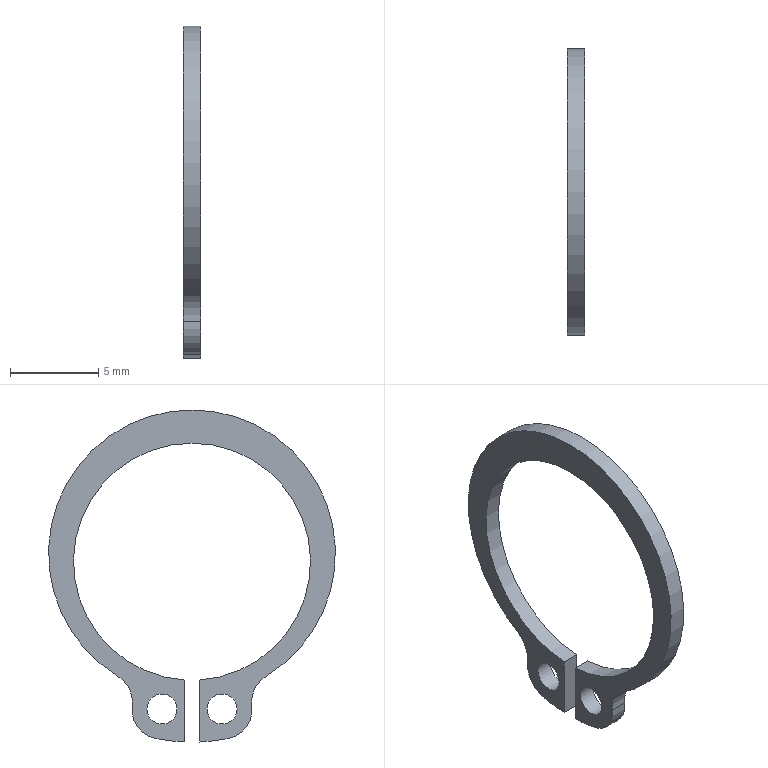Part | NX | features DATUM_CSYS 2, EXTRUDE 1, SKETCH 1 | 1 solid | 14 faces | box 1 x 16.22 x 18.771 mm | volume 75.444 mm3 | cylinder 10 | plane 4 | commonest cylinder face diameters 3.4 x4 1.7 x2 20.4 x2 13.4 x1 16.22 x1
STEP:
#1=CARTESIAN_POINT('',(0.,-4.196,-6.94));
#2=VERTEX_POINT('',#1);
#3=CARTESIAN_POINT('',(0.,-3.388,-8.596));
#4=VERTEX_POINT('',#3);
#5=CARTESIAN_POINT('',(0.,-5.076,-8.395));
#6=DIRECTION('',(-1.,0.,0.));
#7=DIRECTION('',(0.,1.,0.));
#8=AXIS2_PLACEMENT_3D('',#5,#6,#7);
#9=CIRCLE('',#8,1.7);
#10=EDGE_CURVE('',#2,#4,#9,.T.);
#11=ORIENTED_EDGE('',*,*,#10,.T.);
#12=CARTESIAN_POINT('',(1.,-3.388,-8.596));
#13=VERTEX_POINT('',#12);
#14=CARTESIAN_POINT('',(1.,-3.388,-8.596));
#15=DIRECTION('',(-1.,0.,0.));
#16=VECTOR('',#15,1000.);
#17=LINE('',#14,#16);
#18=EDGE_CURVE('',#13,#4,#17,.T.);
#19=ORIENTED_EDGE('',*,*,#18,.F.);
#20=CARTESIAN_POINT('',(1.,-4.196,-6.94));
#21=VERTEX_POINT('',#20);
#22=CARTESIAN_POINT('',(1.,-5.076,-8.395));
#23=DIRECTION('',(-1.,0.,0.));
#24=DIRECTION('',(0.,1.,0.));
#25=AXIS2_PLACEMENT_3D('',#22,#23,#24);
#26=CIRCLE('',#25,1.7);
#27=EDGE_CURVE('',#21,#13,#26,.T.);
#28=ORIENTED_EDGE('',*,*,#27,.F.);
#29=CARTESIAN_POINT('',(1.,-4.196,-6.94));
#30=DIRECTION('',(-1.,0.,0.));
#31=VECTOR('',#30,1000.);
#32=LINE('',#29,#31);
#33=EDGE_CURVE('',#21,#2,#32,.T.);
#34=ORIENTED_EDGE('',*,*,#33,.T.);
#35=EDGE_LOOP('',(#11,#19,#28,#34));
#36=FACE_BOUND('',#35,.T.);
#37=CARTESIAN_POINT('',(1.,-5.076,-8.395));
#38=DIRECTION('',(-1.,0.,0.));
#39=DIRECTION('',(0.,0.,1.));
#40=AXIS2_PLACEMENT_3D('',#37,#38,#39);
#41=CYLINDRICAL_SURFACE('',#40,1.7);
#42=ADVANCED_FACE('',(#36),#41,.F.);
#43=CARTESIAN_POINT('',(0.,-2.04,-10.464));
#44=VERTEX_POINT('',#43);
#45=CARTESIAN_POINT('',(0.,-1.7,-8.798));
#46=DIRECTION('',(1.,0.,0.));
#47=DIRECTION('',(0.,1.,0.));
#48=AXIS2_PLACEMENT_3D('',#45,#46,#47);
#49=CIRCLE('',#48,1.7);
#50=EDGE_CURVE('',#4,#44,#49,.T.);
#51=ORIENTED_EDGE('',*,*,#50,.T.);
#52=CARTESIAN_POINT('',(1.,-2.04,-10.464));
#53=VERTEX_POINT('',#52);
#54=CARTESIAN_POINT('',(1.,-2.04,-10.464));
#55=DIRECTION('',(-1.,0.,0.));
#56=VECTOR('',#55,1000.);
#57=LINE('',#54,#56);
#58=EDGE_CURVE('',#53,#44,#57,.T.);
#59=ORIENTED_EDGE('',*,*,#58,.F.);
#60=CARTESIAN_POINT('',(1.,-1.7,-8.798));
#61=DIRECTION('',(1.,0.,0.));
#62=DIRECTION('',(0.,1.,0.));
#63=AXIS2_PLACEMENT_3D('',#60,#61,#62);
#64=CIRCLE('',#63,1.7);
#65=EDGE_CURVE('',#13,#53,#64,.T.);
#66=ORIENTED_EDGE('',*,*,#65,.F.);
#67=ORIENTED_EDGE('',*,*,#18,.T.);
#68=EDGE_LOOP('',(#51,#59,#66,#67));
#69=FACE_BOUND('',#68,.T.);
#70=CARTESIAN_POINT('',(1.,-1.7,-8.798));
#71=DIRECTION('',(-1.,0.,0.));
#72=DIRECTION('',(0.,0.,1.));
#73=AXIS2_PLACEMENT_3D('',#70,#71,#72);
#74=CYLINDRICAL_SURFACE('',#73,1.7);
#75=ADVANCED_FACE('',(#69),#74,.T.);
#76=CARTESIAN_POINT('',(0.,-0.425,-10.661));
#77=VERTEX_POINT('',#76);
#78=CARTESIAN_POINT('',(0.,0.,-0.47));
#79=DIRECTION('',(1.,0.,0.));
#80=DIRECTION('',(0.,1.,0.));
#81=AXIS2_PLACEMENT_3D('',#78,#79,#80);
#82=CIRCLE('',#81,10.2);
#83=EDGE_CURVE('',#44,#77,#82,.T.);
#84=ORIENTED_EDGE('',*,*,#83,.T.);
#85=CARTESIAN_POINT('',(1.,-0.425,-10.661));
#86=VERTEX_POINT('',#85);
#87=CARTESIAN_POINT('',(1.,-0.425,-10.661));
#88=DIRECTION('',(-1.,0.,0.));
#89=VECTOR('',#88,1000.);
#90=LINE('',#87,#89);
#91=EDGE_CURVE('',#86,#77,#90,.T.);
#92=ORIENTED_EDGE('',*,*,#91,.F.);
#93=CARTESIAN_POINT('',(1.,0.,-0.47));
#94=DIRECTION('',(1.,0.,0.));
#95=DIRECTION('',(0.,1.,0.));
#96=AXIS2_PLACEMENT_3D('',#93,#94,#95);
#97=CIRCLE('',#96,10.2);
#98=EDGE_CURVE('',#53,#86,#97,.T.);
#99=ORIENTED_EDGE('',*,*,#98,.F.);
#100=ORIENTED_EDGE('',*,*,#58,.T.);
#101=EDGE_LOOP('',(#84,#92,#99,#100));
#102=FACE_BOUND('',#101,.T.);
#103=CARTESIAN_POINT('',(1.,0.,-0.47));
#104=DIRECTION('',(-1.,0.,0.));
#105=DIRECTION('',(0.,0.,1.));
#106=AXIS2_PLACEMENT_3D('',#103,#104,#105);
#107=CYLINDRICAL_SURFACE('',#106,10.2);
#108=ADVANCED_FACE('',(#102),#107,.T.);
#109=CARTESIAN_POINT('',(0.,-0.425,-7.157));
#110=VERTEX_POINT('',#109);
#111=CARTESIAN_POINT('',(0.,-0.425,-10.661));
#112=DIRECTION('',(0.,0.,1.));
#113=VECTOR('',#112,1000.);
#114=LINE('',#111,#113);
#115=EDGE_CURVE('',#77,#110,#114,.T.);
#116=ORIENTED_EDGE('',*,*,#115,.T.);
#117=CARTESIAN_POINT('',(1.,-0.425,-7.157));
#118=VERTEX_POINT('',#117);
#119=CARTESIAN_POINT('',(1.,-0.425,-7.157));
#120=DIRECTION('',(-1.,0.,0.));
#121=VECTOR('',#120,1000.);
#122=LINE('',#119,#121);
#123=EDGE_CURVE('',#118,#110,#122,.T.);
#124=ORIENTED_EDGE('',*,*,#123,.F.);
#125=CARTESIAN_POINT('',(1.,-0.425,-10.661));
#126=DIRECTION('',(0.,0.,1.));
#127=VECTOR('',#126,1000.);
#128=LINE('',#125,#127);
#129=EDGE_CURVE('',#86,#118,#128,.T.);
#130=ORIENTED_EDGE('',*,*,#129,.F.);
#131=ORIENTED_EDGE('',*,*,#91,.T.);
#132=EDGE_LOOP('',(#116,#124,#130,#131));
#133=FACE_BOUND('',#132,.T.);
#134=CARTESIAN_POINT('',(1.,-0.425,-10.661));
#135=DIRECTION('',(0.,-1.,0.));
#136=DIRECTION('',(0.,0.,-1.));
#137=AXIS2_PLACEMENT_3D('',#134,#135,#136);
#138=PLANE('',#137);
#139=ADVANCED_FACE('',(#133),#138,.F.);
#140=CARTESIAN_POINT('',(0.,0.425,-7.157));
#141=VERTEX_POINT('',#140);
#142=CARTESIAN_POINT('',(0.,0.,-0.47));
#143=DIRECTION('',(-1.,0.,0.));
#144=DIRECTION('',(0.,1.,0.));
#145=AXIS2_PLACEMENT_3D('',#142,#143,#144);
#146=CIRCLE('',#145,6.7);
#147=EDGE_CURVE('',#110,#141,#146,.T.);
#148=ORIENTED_EDGE('',*,*,#147,.T.);
#149=CARTESIAN_POINT('',(1.,0.425,-7.157));
#150=VERTEX_POINT('',#149);
#151=CARTESIAN_POINT('',(1.,0.425,-7.157));
#152=DIRECTION('',(-1.,0.,0.));
#153=VECTOR('',#152,1000.);
#154=LINE('',#151,#153);
#155=EDGE_CURVE('',#150,#141,#154,.T.);
#156=ORIENTED_EDGE('',*,*,#155,.F.);
#157=CARTESIAN_POINT('',(1.,0.,-0.47));
#158=DIRECTION('',(-1.,0.,0.));
#159=DIRECTION('',(0.,1.,0.));
#160=AXIS2_PLACEMENT_3D('',#157,#158,#159);
#161=CIRCLE('',#160,6.7);
#162=EDGE_CURVE('',#118,#150,#161,.T.);
#163=ORIENTED_EDGE('',*,*,#162,.F.);
#164=ORIENTED_EDGE('',*,*,#123,.T.);
#165=EDGE_LOOP('',(#148,#156,#163,#164));
#166=FACE_BOUND('',#165,.T.);
#167=CARTESIAN_POINT('',(1.,0.,-0.47));
#168=DIRECTION('',(-1.,0.,0.));
#169=DIRECTION('',(0.,0.,1.));
#170=AXIS2_PLACEMENT_3D('',#167,#168,#169);
#171=CYLINDRICAL_SURFACE('',#170,6.7);
#172=ADVANCED_FACE('',(#166),#171,.F.);
#173=CARTESIAN_POINT('',(0.,0.425,-10.661));
#174=VERTEX_POINT('',#173);
#175=CARTESIAN_POINT('',(0.,0.425,-7.157));
#176=DIRECTION('',(0.,0.,-1.));
#177=VECTOR('',#176,1000.);
#178=LINE('',#175,#177);
#179=EDGE_CURVE('',#141,#174,#178,.T.);
#180=ORIENTED_EDGE('',*,*,#179,.T.);
#181=CARTESIAN_POINT('',(1.,0.425,-10.661));
#182=VERTEX_POINT('',#181);
#183=CARTESIAN_POINT('',(1.,0.425,-10.661));
#184=DIRECTION('',(-1.,0.,0.));
#185=VECTOR('',#184,1000.);
#186=LINE('',#183,#185);
#187=EDGE_CURVE('',#182,#174,#186,.T.);
#188=ORIENTED_EDGE('',*,*,#187,.F.);
#189=CARTESIAN_POINT('',(1.,0.425,-7.157));
#190=DIRECTION('',(0.,0.,-1.));
#191=VECTOR('',#190,1000.);
#192=LINE('',#189,#191);
#193=EDGE_CURVE('',#150,#182,#192,.T.);
#194=ORIENTED_EDGE('',*,*,#193,.F.);
#195=ORIENTED_EDGE('',*,*,#155,.T.);
#196=EDGE_LOOP('',(#180,#188,#194,#195));
#197=FACE_BOUND('',#196,.T.);
#198=CARTESIAN_POINT('',(1.,0.425,-7.157));
#199=DIRECTION('',(0.,1.,0.));
#200=DIRECTION('',(0.,0.,1.));
#201=AXIS2_PLACEMENT_3D('',#198,#199,#200);
#202=PLANE('',#201);
#203=ADVANCED_FACE('',(#197),#202,.F.);
#204=CARTESIAN_POINT('',(0.,2.04,-10.464));
#205=VERTEX_POINT('',#204);
#206=CARTESIAN_POINT('',(0.,0.,-0.47));
#207=DIRECTION('',(1.,0.,0.));
#208=DIRECTION('',(0.,1.,0.));
#209=AXIS2_PLACEMENT_3D('',#206,#207,#208);
#210=CIRCLE('',#209,10.2);
#211=EDGE_CURVE('',#174,#205,#210,.T.);
#212=ORIENTED_EDGE('',*,*,#211,.T.);
#213=CARTESIAN_POINT('',(1.,2.04,-10.464));
#214=VERTEX_POINT('',#213);
#215=CARTESIAN_POINT('',(1.,2.04,-10.464));
#216=DIRECTION('',(-1.,0.,0.));
#217=VECTOR('',#216,1000.);
#218=LINE('',#215,#217);
#219=EDGE_CURVE('',#214,#205,#218,.T.);
#220=ORIENTED_EDGE('',*,*,#219,.F.);
#221=CARTESIAN_POINT('',(1.,0.,-0.47));
#222=DIRECTION('',(1.,0.,0.));
#223=DIRECTION('',(0.,1.,0.));
#224=AXIS2_PLACEMENT_3D('',#221,#222,#223);
#225=CIRCLE('',#224,10.2);
#226=EDGE_CURVE('',#182,#214,#225,.T.);
#227=ORIENTED_EDGE('',*,*,#226,.F.);
#228=ORIENTED_EDGE('',*,*,#187,.T.);
#229=EDGE_LOOP('',(#212,#220,#227,#228));
#230=FACE_BOUND('',#229,.T.);
#231=CARTESIAN_POINT('',(1.,0.,-0.47));
#232=DIRECTION('',(-1.,0.,0.));
#233=DIRECTION('',(0.,0.,1.));
#234=AXIS2_PLACEMENT_3D('',#231,#232,#233);
#235=CYLINDRICAL_SURFACE('',#234,10.2);
#236=ADVANCED_FACE('',(#230),#235,.T.);
#237=CARTESIAN_POINT('',(0.,3.388,-8.596));
#238=VERTEX_POINT('',#237);
#239=CARTESIAN_POINT('',(0.,1.7,-8.798));
#240=DIRECTION('',(1.,0.,0.));
#241=DIRECTION('',(0.,-1.,0.));
#242=AXIS2_PLACEMENT_3D('',#239,#240,#241);
#243=CIRCLE('',#242,1.7);
#244=EDGE_CURVE('',#205,#238,#243,.T.);
#245=ORIENTED_EDGE('',*,*,#244,.T.);
#246=CARTESIAN_POINT('',(1.,3.388,-8.596));
#247=VERTEX_POINT('',#246);
#248=CARTESIAN_POINT('',(1.,3.388,-8.596));
#249=DIRECTION('',(-1.,0.,0.));
#250=VECTOR('',#249,1000.);
#251=LINE('',#248,#250);
#252=EDGE_CURVE('',#247,#238,#251,.T.);
#253=ORIENTED_EDGE('',*,*,#252,.F.);
#254=CARTESIAN_POINT('',(1.,1.7,-8.798));
#255=DIRECTION('',(1.,0.,0.));
#256=DIRECTION('',(0.,-1.,0.));
#257=AXIS2_PLACEMENT_3D('',#254,#255,#256);
#258=CIRCLE('',#257,1.7);
#259=EDGE_CURVE('',#214,#247,#258,.T.);
#260=ORIENTED_EDGE('',*,*,#259,.F.);
#261=ORIENTED_EDGE('',*,*,#219,.T.);
#262=EDGE_LOOP('',(#245,#253,#260,#261));
#263=FACE_BOUND('',#262,.T.);
#264=CARTESIAN_POINT('',(1.,1.7,-8.798));
#265=DIRECTION('',(-1.,0.,0.));
#266=DIRECTION('',(0.,0.,1.));
#267=AXIS2_PLACEMENT_3D('',#264,#265,#266);
#268=CYLINDRICAL_SURFACE('',#267,1.7);
#269=ADVANCED_FACE('',(#263),#268,.T.);
#270=CARTESIAN_POINT('',(0.,4.196,-6.94));
#271=VERTEX_POINT('',#270);
#272=CARTESIAN_POINT('',(0.,5.076,-8.395));
#273=DIRECTION('',(-1.,0.,0.));
#274=DIRECTION('',(0.,-1.,0.));
#275=AXIS2_PLACEMENT_3D('',#272,#273,#274);
#276=CIRCLE('',#275,1.7);
#277=EDGE_CURVE('',#238,#271,#276,.T.);
#278=ORIENTED_EDGE('',*,*,#277,.T.);
#279=CARTESIAN_POINT('',(1.,4.196,-6.94));
#280=VERTEX_POINT('',#279);
#281=CARTESIAN_POINT('',(1.,4.196,-6.94));
#282=DIRECTION('',(-1.,0.,0.));
#283=VECTOR('',#282,1000.);
#284=LINE('',#281,#283);
#285=EDGE_CURVE('',#280,#271,#284,.T.);
#286=ORIENTED_EDGE('',*,*,#285,.F.);
#287=CARTESIAN_POINT('',(1.,5.076,-8.395));
#288=DIRECTION('',(-1.,0.,0.));
#289=DIRECTION('',(0.,-1.,0.));
#290=AXIS2_PLACEMENT_3D('',#287,#288,#289);
#291=CIRCLE('',#290,1.7);
#292=EDGE_CURVE('',#247,#280,#291,.T.);
#293=ORIENTED_EDGE('',*,*,#292,.F.);
#294=ORIENTED_EDGE('',*,*,#252,.T.);
#295=EDGE_LOOP('',(#278,#286,#293,#294));
#296=FACE_BOUND('',#295,.T.);
#297=CARTESIAN_POINT('',(1.,5.076,-8.395));
#298=DIRECTION('',(-1.,0.,0.));
#299=DIRECTION('',(0.,0.,1.));
#300=AXIS2_PLACEMENT_3D('',#297,#298,#299);
#301=CYLINDRICAL_SURFACE('',#300,1.7);
#302=ADVANCED_FACE('',(#296),#301,.F.);
#303=CARTESIAN_POINT('',(1.,-0.85,-8.798));
#304=VERTEX_POINT('',#303);
#305=CARTESIAN_POINT('',(1.,-1.7,-8.798));
#306=DIRECTION('',(1.,0.,0.));
#307=DIRECTION('',(0.,1.,0.));
#308=AXIS2_PLACEMENT_3D('',#305,#306,#307);
#309=CIRCLE('',#308,0.85);
#310=EDGE_CURVE('',#304,#304,#309,.T.);
#311=ORIENTED_EDGE('',*,*,#310,.T.);
#312=EDGE_LOOP('',(#311));
#313=FACE_BOUND('',#312,.T.);
#314=CARTESIAN_POINT('',(0.,-0.85,-8.798));
#315=VERTEX_POINT('',#314);
#316=CARTESIAN_POINT('',(0.,-1.7,-8.798));
#317=DIRECTION('',(1.,0.,0.));
#318=DIRECTION('',(0.,1.,0.));
#319=AXIS2_PLACEMENT_3D('',#316,#317,#318);
#320=CIRCLE('',#319,0.85);
#321=EDGE_CURVE('',#315,#315,#320,.T.);
#322=ORIENTED_EDGE('',*,*,#321,.F.);
#323=EDGE_LOOP('',(#322));
#324=FACE_BOUND('',#323,.T.);
#325=CARTESIAN_POINT('',(1.,-1.7,-8.798));
#326=DIRECTION('',(-1.,0.,0.));
#327=DIRECTION('',(0.,0.,1.));
#328=AXIS2_PLACEMENT_3D('',#325,#326,#327);
#329=CYLINDRICAL_SURFACE('',#328,0.85);
#330=ADVANCED_FACE('',(#313,#324),#329,.F.);
#331=CARTESIAN_POINT('',(0.,0.,0.));
#332=DIRECTION('',(1.,0.,0.));
#333=DIRECTION('',(0.,1.,0.));
#334=AXIS2_PLACEMENT_3D('',#331,#332,#333);
#335=CIRCLE('',#334,8.11);
#336=EDGE_CURVE('',#271,#2,#335,.T.);
#337=ORIENTED_EDGE('',*,*,#336,.T.);
#338=ORIENTED_EDGE('',*,*,#33,.F.);
#339=CARTESIAN_POINT('',(1.,0.,0.));
#340=DIRECTION('',(1.,0.,0.));
#341=DIRECTION('',(0.,1.,0.));
#342=AXIS2_PLACEMENT_3D('',#339,#340,#341);
#343=CIRCLE('',#342,8.11);
#344=EDGE_CURVE('',#280,#21,#343,.T.);
#345=ORIENTED_EDGE('',*,*,#344,.F.);
#346=ORIENTED_EDGE('',*,*,#285,.T.);
#347=EDGE_LOOP('',(#337,#338,#345,#346));
#348=FACE_BOUND('',#347,.T.);
#349=CARTESIAN_POINT('',(1.,0.,0.));
#350=DIRECTION('',(-1.,0.,0.));
#351=DIRECTION('',(0.,0.,1.));
#352=AXIS2_PLACEMENT_3D('',#349,#350,#351);
#353=CYLINDRICAL_SURFACE('',#352,8.11);
#354=ADVANCED_FACE('',(#348),#353,.T.);
#355=CARTESIAN_POINT('',(1.,2.55,-8.798));
#356=VERTEX_POINT('',#355);
#357=CARTESIAN_POINT('',(1.,1.7,-8.798));
#358=DIRECTION('',(1.,0.,0.));
#359=DIRECTION('',(0.,1.,0.));
#360=AXIS2_PLACEMENT_3D('',#357,#358,#359);
#361=CIRCLE('',#360,0.85);
#362=EDGE_CURVE('',#356,#356,#361,.T.);
#363=ORIENTED_EDGE('',*,*,#362,.T.);
#364=EDGE_LOOP('',(#363));
#365=FACE_BOUND('',#364,.T.);
#366=CARTESIAN_POINT('',(0.,2.55,-8.798));
#367=VERTEX_POINT('',#366);
#368=CARTESIAN_POINT('',(0.,1.7,-8.798));
#369=DIRECTION('',(1.,0.,0.));
#370=DIRECTION('',(0.,1.,0.));
#371=AXIS2_PLACEMENT_3D('',#368,#369,#370);
#372=CIRCLE('',#371,0.85);
#373=EDGE_CURVE('',#367,#367,#372,.T.);
#374=ORIENTED_EDGE('',*,*,#373,.F.);
#375=EDGE_LOOP('',(#374));
#376=FACE_BOUND('',#375,.T.);
#377=CARTESIAN_POINT('',(1.,1.7,-8.798));
#378=DIRECTION('',(-1.,0.,0.));
#379=DIRECTION('',(0.,0.,1.));
#380=AXIS2_PLACEMENT_3D('',#377,#378,#379);
#381=CYLINDRICAL_SURFACE('',#380,0.85);
#382=ADVANCED_FACE('',(#365,#376),#381,.F.);
#383=ORIENTED_EDGE('',*,*,#27,.T.);
#384=ORIENTED_EDGE('',*,*,#65,.T.);
#385=ORIENTED_EDGE('',*,*,#98,.T.);
#386=ORIENTED_EDGE('',*,*,#129,.T.);
#387=ORIENTED_EDGE('',*,*,#162,.T.);
#388=ORIENTED_EDGE('',*,*,#193,.T.);
#389=ORIENTED_EDGE('',*,*,#226,.T.);
#390=ORIENTED_EDGE('',*,*,#259,.T.);
#391=ORIENTED_EDGE('',*,*,#292,.T.);
#392=ORIENTED_EDGE('',*,*,#344,.T.);
#393=EDGE_LOOP('',(#383,#384,#385,#386,#387,#388,#389,#390,#391,#392));
#394=FACE_BOUND('',#393,.T.);
#395=ORIENTED_EDGE('',*,*,#310,.F.);
#396=EDGE_LOOP('',(#395));
#397=FACE_BOUND('',#396,.T.);
#398=ORIENTED_EDGE('',*,*,#362,.F.);
#399=EDGE_LOOP('',(#398));
#400=FACE_BOUND('',#399,.T.);
#401=CARTESIAN_POINT('',(1.,-5.076,-8.395));
#402=DIRECTION('',(-1.,0.,0.));
#403=DIRECTION('',(0.,0.,1.));
#404=AXIS2_PLACEMENT_3D('',#401,#402,#403);
#405=PLANE('',#404);
#406=ADVANCED_FACE('',(#394,#397,#400),#405,.F.);
#407=ORIENTED_EDGE('',*,*,#10,.F.);
#408=ORIENTED_EDGE('',*,*,#336,.F.);
#409=ORIENTED_EDGE('',*,*,#277,.F.);
#410=ORIENTED_EDGE('',*,*,#244,.F.);
#411=ORIENTED_EDGE('',*,*,#211,.F.);
#412=ORIENTED_EDGE('',*,*,#179,.F.);
#413=ORIENTED_EDGE('',*,*,#147,.F.);
#414=ORIENTED_EDGE('',*,*,#115,.F.);
#415=ORIENTED_EDGE('',*,*,#83,.F.);
#416=ORIENTED_EDGE('',*,*,#50,.F.);
#417=EDGE_LOOP('',(#407,#408,#409,#410,#411,#412,#413,#414,#415,#416));
#418=FACE_BOUND('',#417,.T.);
#419=ORIENTED_EDGE('',*,*,#321,.T.);
#420=EDGE_LOOP('',(#419));
#421=FACE_BOUND('',#420,.T.);
#422=ORIENTED_EDGE('',*,*,#373,.T.);
#423=EDGE_LOOP('',(#422));
#424=FACE_BOUND('',#423,.T.);
#425=CARTESIAN_POINT('',(0.,-5.076,-8.395));
#426=DIRECTION('',(-1.,0.,0.));
#427=DIRECTION('',(0.,0.,1.));
#428=AXIS2_PLACEMENT_3D('',#425,#426,#427);
#429=PLANE('',#428);
#430=ADVANCED_FACE('',(#418,#421,#424),#429,.T.);
#431=CLOSED_SHELL('',(#42,#75,#108,#139,#172,#203,#236,#269,#302,#330,#354,#382,#406,#430));
#432=MANIFOLD_SOLID_BREP('',#431);
#433=(LENGTH_UNIT()NAMED_UNIT(*)SI_UNIT(.MILLI.,.METRE.));
#434=UNCERTAINTY_MEASURE_WITH_UNIT(LENGTH_MEASURE(0.00001),#433,'','');
#435=(NAMED_UNIT(*)PLANE_ANGLE_UNIT()SI_UNIT($,.RADIAN.));
#436=(NAMED_UNIT(*)SI_UNIT($,.STERADIAN.)SOLID_ANGLE_UNIT());
#437=(GEOMETRIC_REPRESENTATION_CONTEXT(3)GLOBAL_UNCERTAINTY_ASSIGNED_CONTEXT((#434))GLOBAL_UNIT_ASSIGNED_CONTEXT((#433,#435,#436))REPRESENTATION_CONTEXT('',''));
#438=ADVANCED_BREP_SHAPE_REPRESENTATION('',(#432),#437);